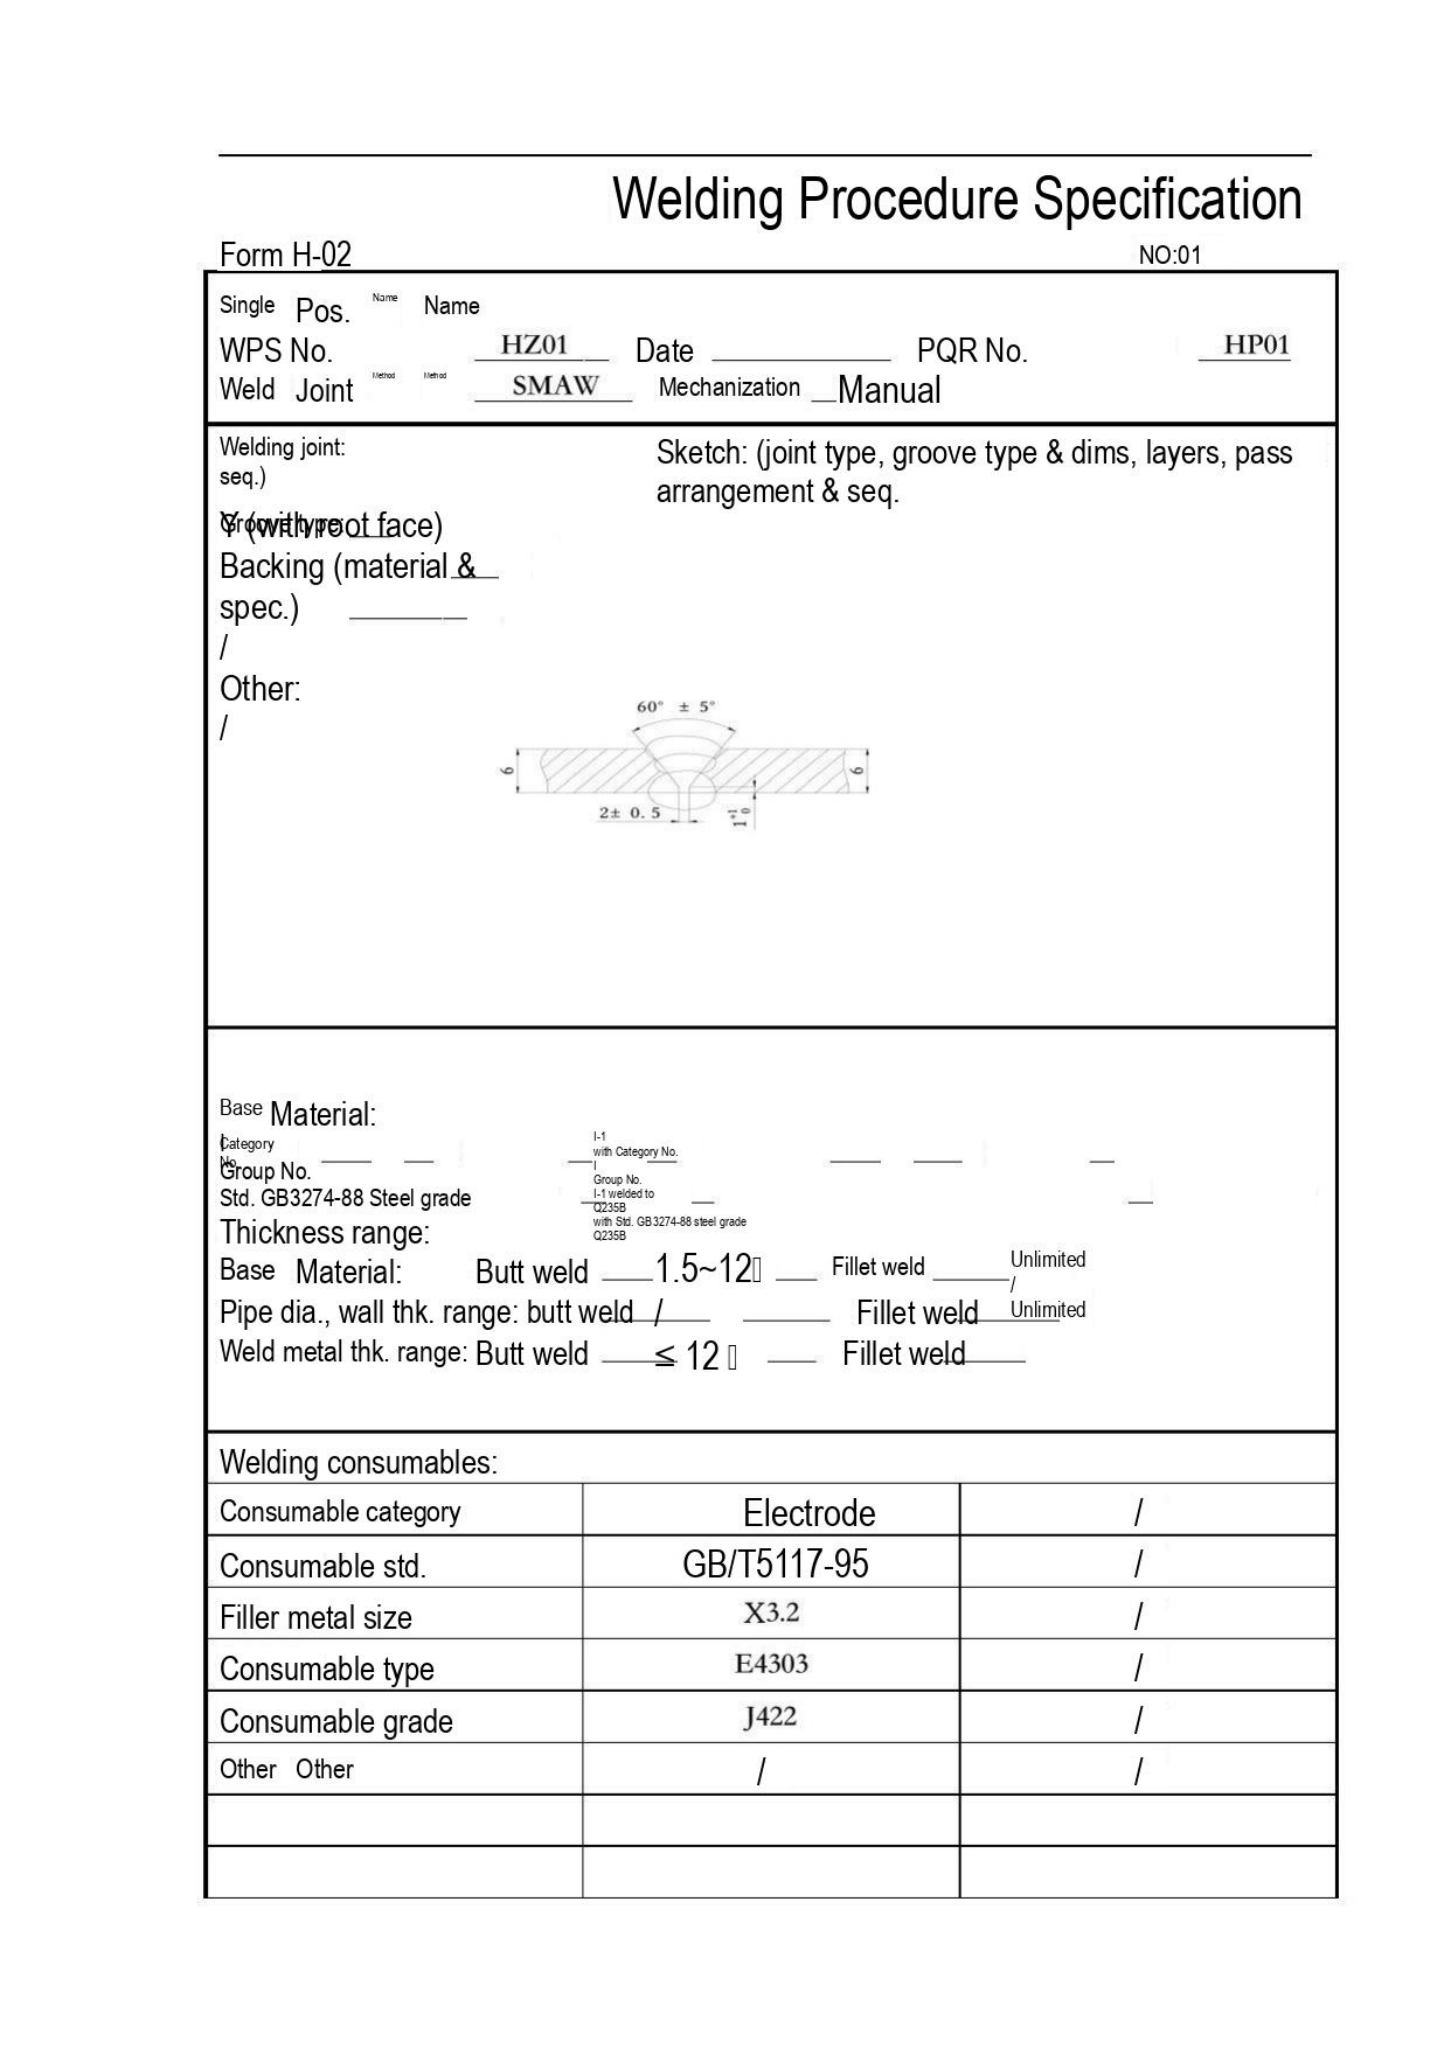Welding Procedure Specification

Form H-02 NO:01

Single Pos. Name Name
WPS No. HZ01 Date PQR No. HP01
Weld Joint Method Method SMAW Mechanization Manual

Welding joint: Sketch: (joint type, groove type & dims, layers, pass arrangement & seq.)
seq.)
Groove type: Y (with root face)
Backing (material & spec.)
/
Other:
/

60° ± 5°
9
9
2± 0.5
1±0

Base Material:
Category No. I-1 with Category No. I
Group No. Group No. I-1 welded to Q235B
Std. GB3274-88 Steel grade with Std. GB3274-88 steel grade Q235B
Thickness range:
Base Material: Butt weld 1.5~12 Fillet weld Unlimited
/
Pipe dia., wall thk. range: butt weld / Fillet weld Unlimited
Weld metal thk. range: Butt weld ≤ 12 Fillet weld

Welding consumables:

| Consumable category | Electrode | / |
|---|---|---|
| Consumable std. | GB/T5117-95 | / |
| Filler metal size | X3.2 | / |
| Consumable type | E4303 | / |
| Consumable grade | J422 | / |
| Other Other | / | / |
| | | |
| | | |
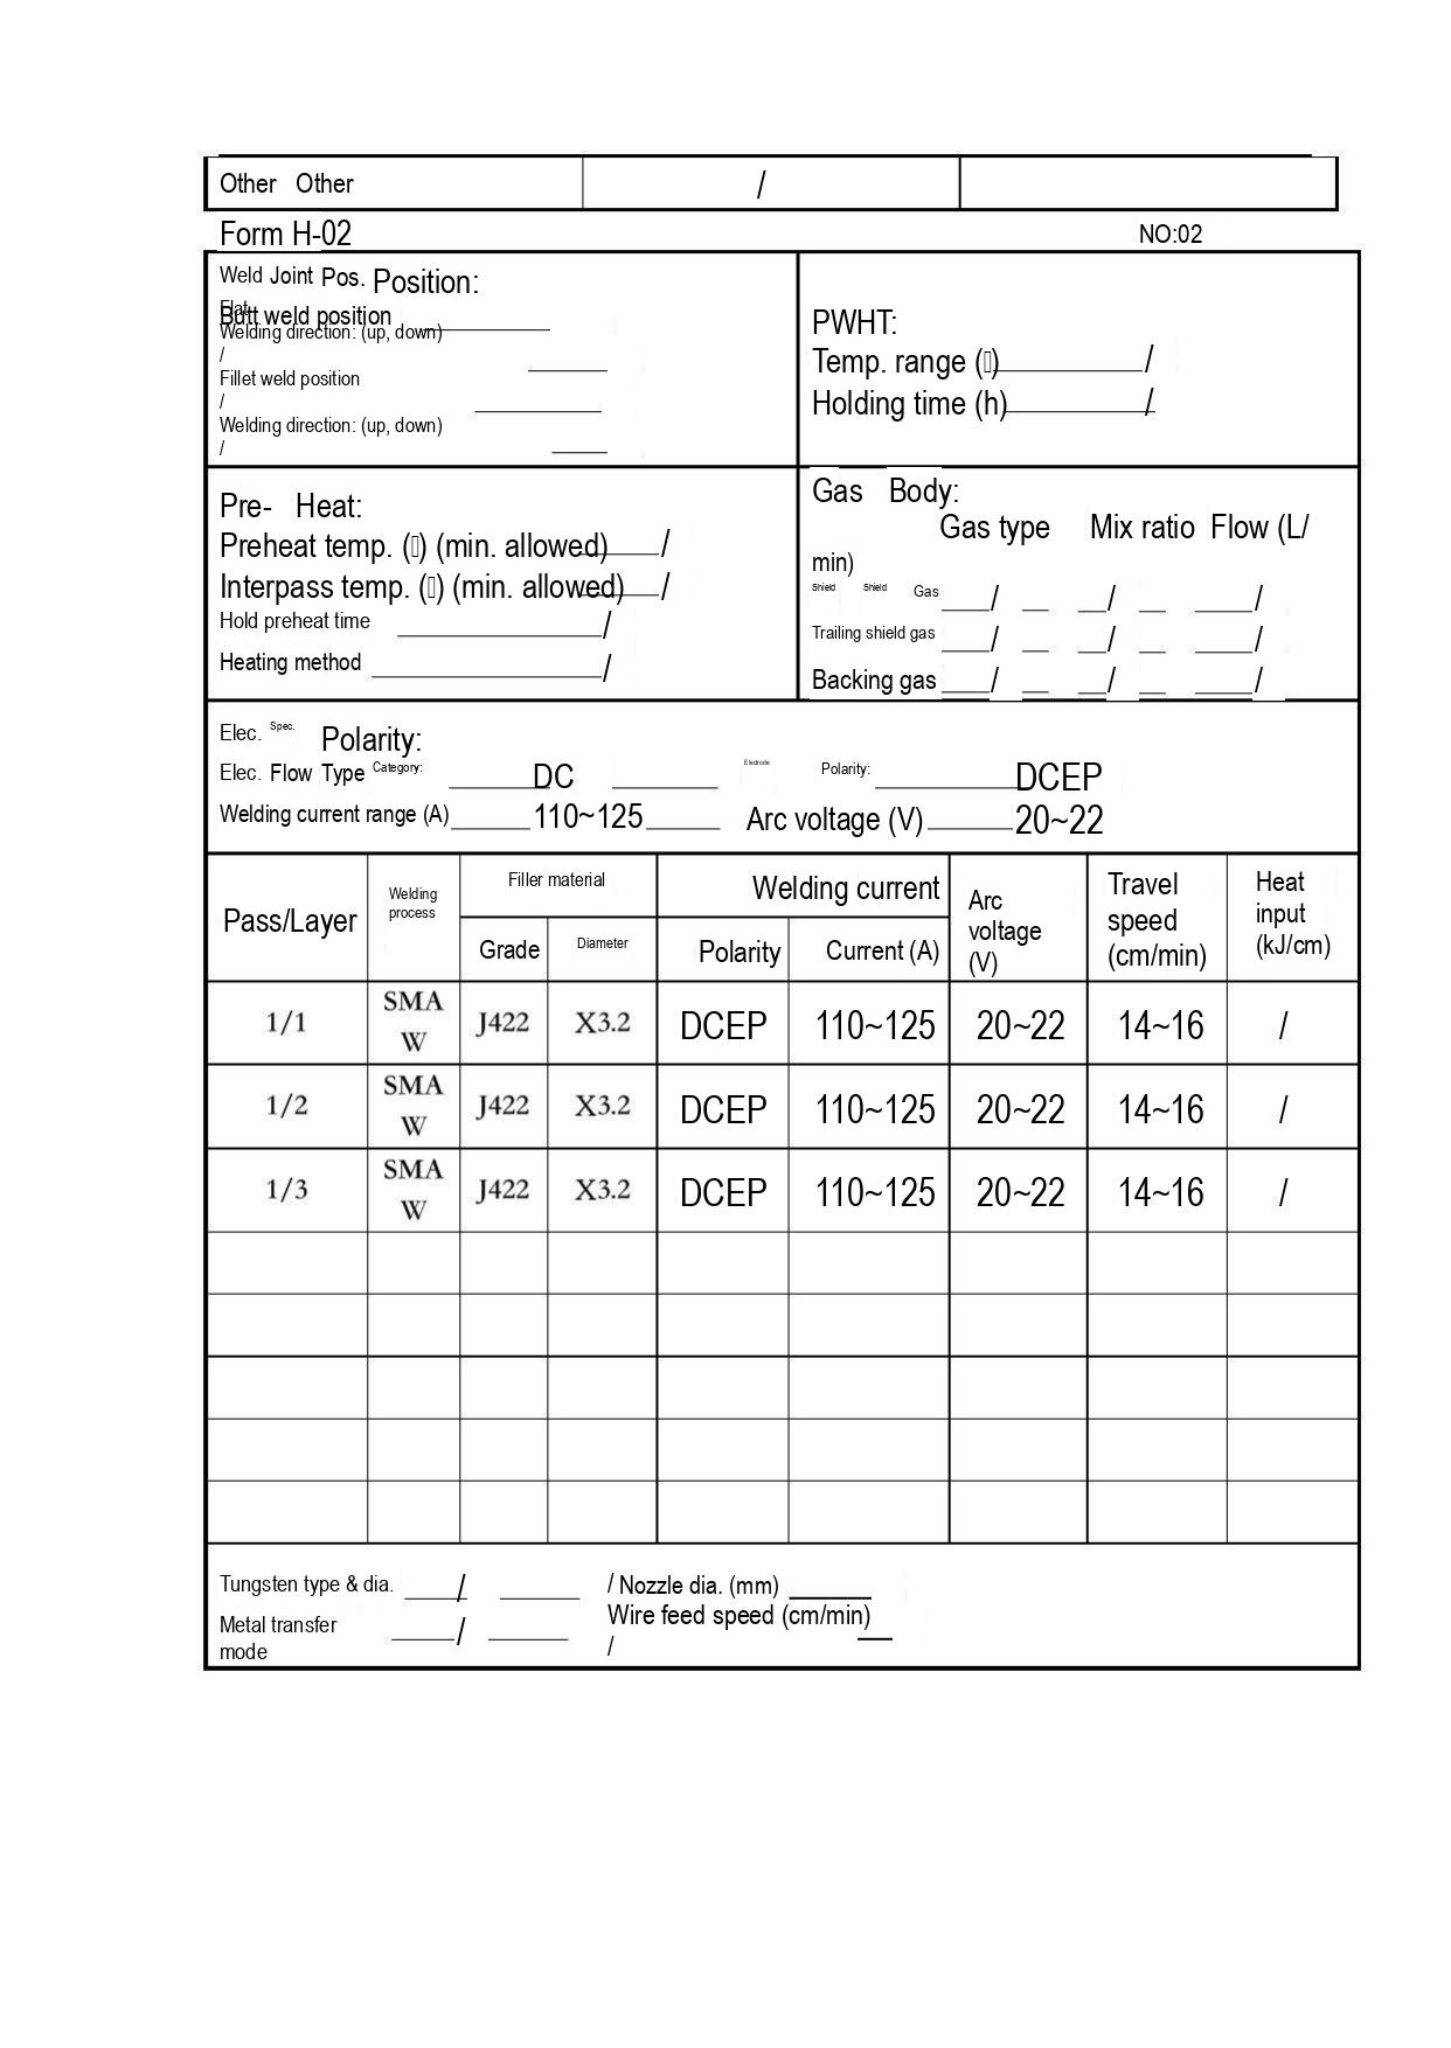| Other Other | / | |
|---|---|---|

Form H-02 NO:02

| Weld Joint Pos. Position:<br>Flat<br>Butt weld position<br>Welding direction: (up, down)<br>/<br>Fillet weld position<br>/<br>Welding direction: (up, down)<br>/ | PWHT:<br>Temp. range (℃) /<br>Holding time (h) / |
|---|---|
| Pre- Heat:<br>Preheat temp. (℃) (min. allowed) /<br>Interpass temp. (℃) (min. allowed) /<br>Hold preheat time /<br>Heating method / | Gas Body:<br>Gas type Mix ratio Flow (L/min)<br>Shield Shield Gas / / /<br>Trailing shield gas / / /<br>Backing gas / / / |

Elec. Spec. Polarity:
Elec. Flow Type Category: DC Electrode Polarity: DCEP
Welding current range (A) 110~125 Arc voltage (V) 20~22

| Pass/Layer | Welding process | Filler material Grade | Filler material Diameter | Welding current Polarity | Welding current Current (A) | Arc voltage (V) | Travel speed (cm/min) | Heat input (kJ/cm) |
|---|---|---|---|---|---|---|---|---|
| 1/1 | SMAW | J422 | X3.2 | DCEP | 110~125 | 20~22 | 14~16 | / |
| 1/2 | SMAW | J422 | X3.2 | DCEP | 110~125 | 20~22 | 14~16 | / |
| 1/3 | SMAW | J422 | X3.2 | DCEP | 110~125 | 20~22 | 14~16 | / |
| | | | | | | | | |
| | | | | | | | | |
| | | | | | | | | |
| | | | | | | | | |
| | | | | | | | | |

Tungsten type & dia. / / Nozzle dia. (mm)
Metal transfer mode / Wire feed speed (cm/min) /
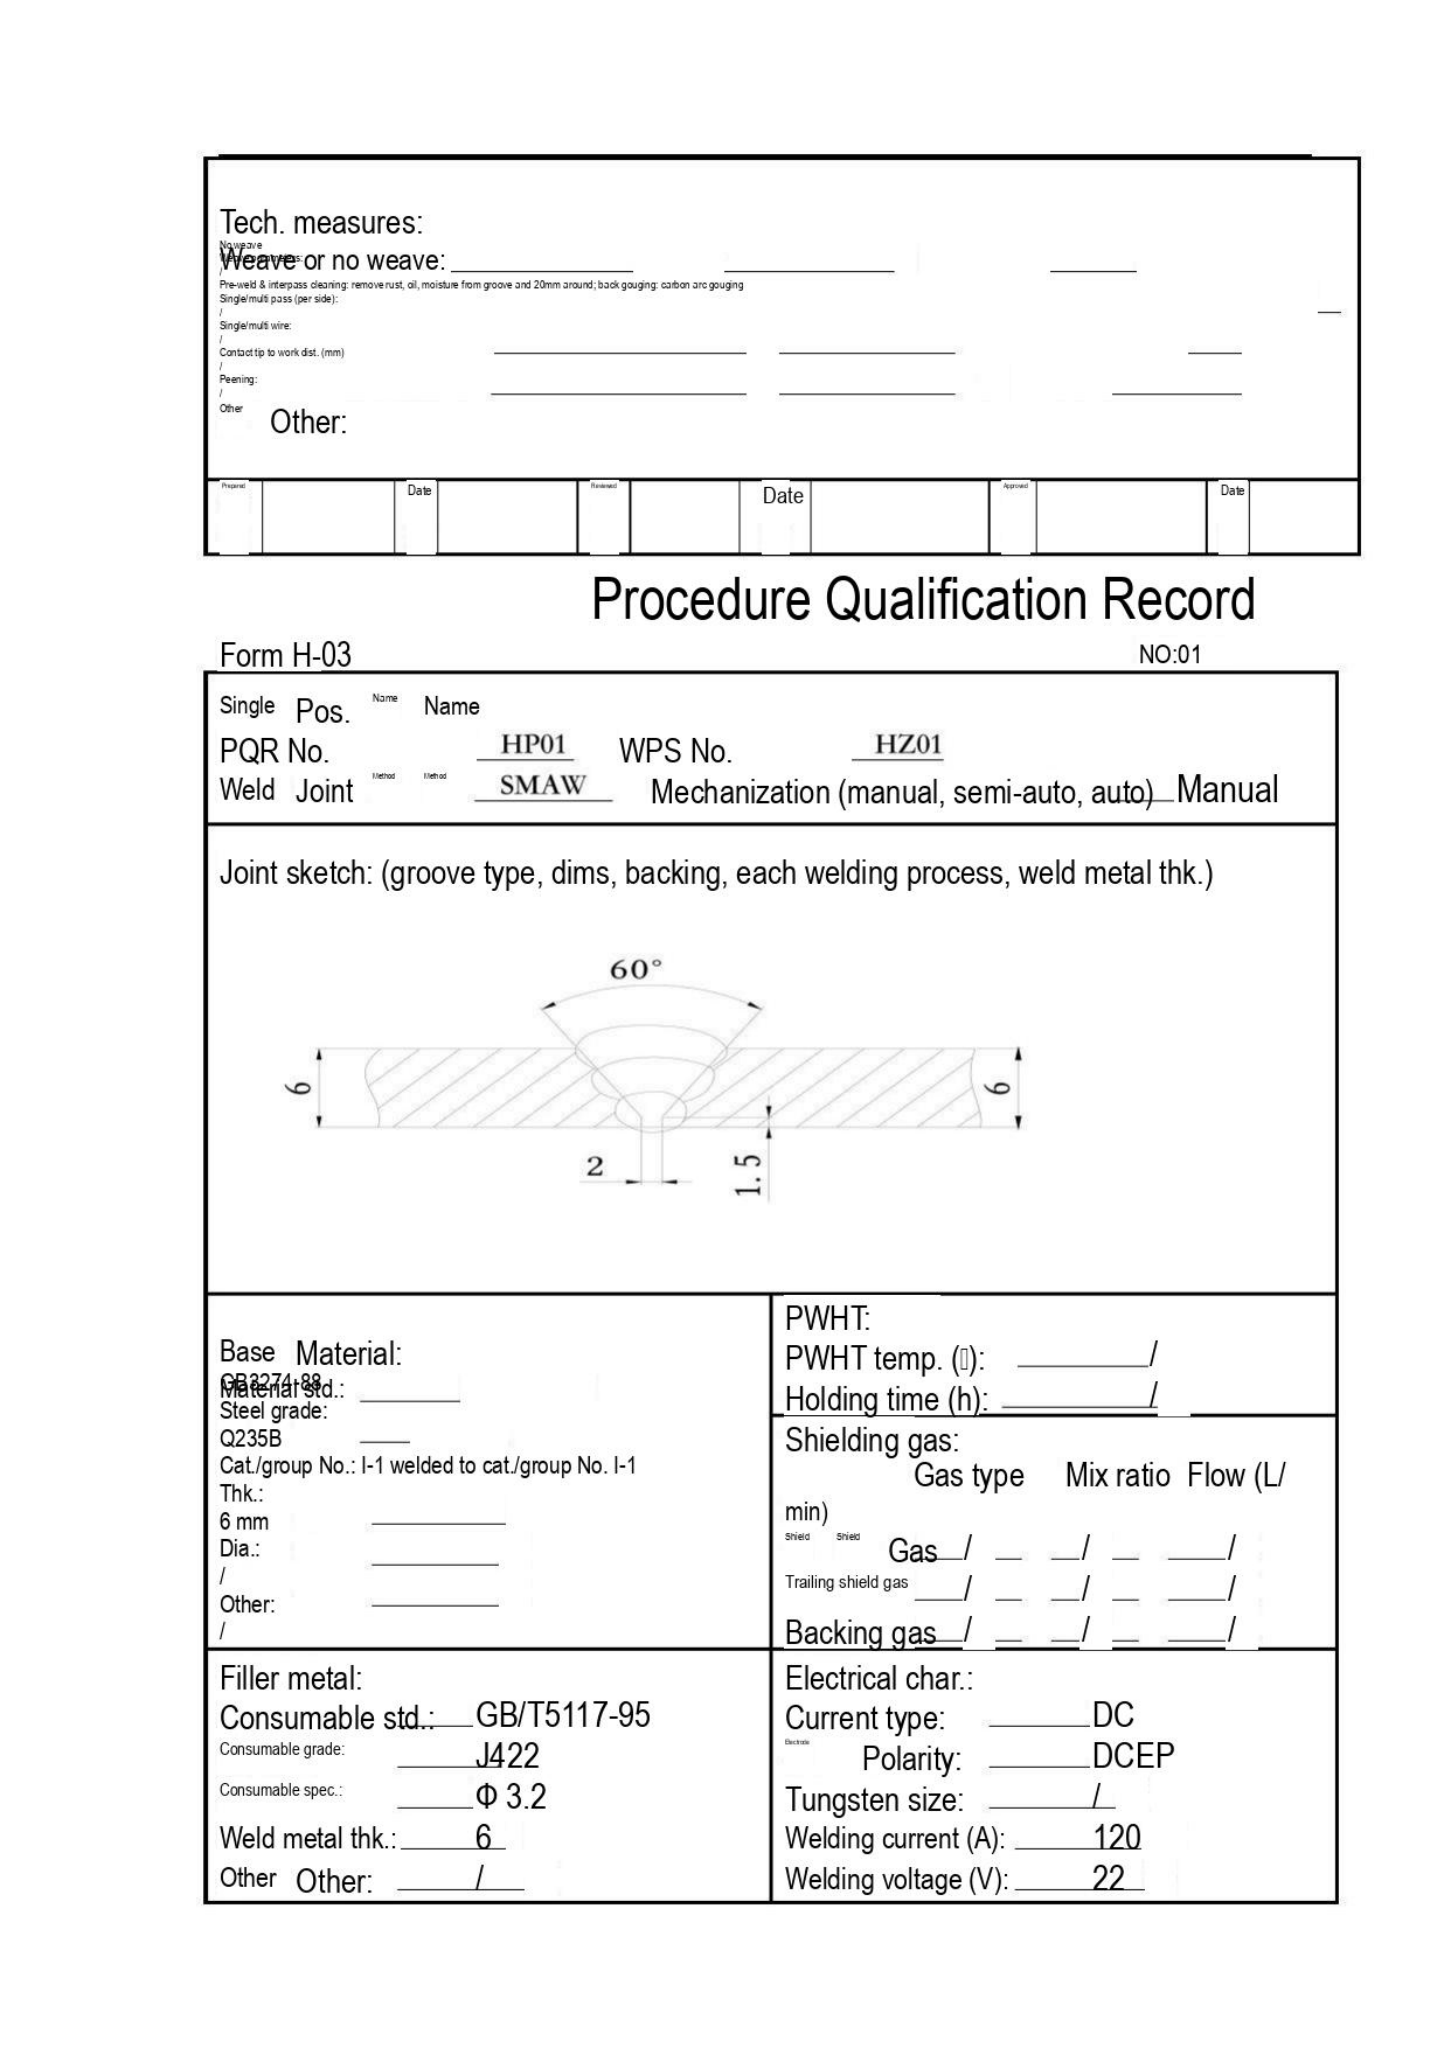Tech. measures:
No weave
Weave or no weave:
Pre-weld & interpass cleaning: remove rust, oil, moisture from groove and 20mm around; back gouging: carbon arc gouging
Single/multi pass (per side):
/
Single/multi wire:
/
Contact tip to work dist. (mm)
/
Peening:
/
Other
Other:

| Prepared | | Date | | Reviewed | | Date | | Approved | | Date | |
|---|---|---|---|---|---|---|---|---|---|---|---|

Procedure Qualification Record

Form H-03 NO:01

Single Pos. Name Name
PQR No. HP01 WPS No. HZ01
Weld Joint Method Method SMAW Mechanization (manual, semi-auto, auto) Manual

Joint sketch: (groove type, dims, backing, each welding process, weld metal thk.)

60°
6
6
2
1.5

| Base Material:<br>GB3274-88<br>Material std.:<br>Steel grade:<br>Q235B<br>Cat./group No.: I-1 welded to cat./group No. I-1<br>Thk.:<br>6 mm<br>Dia.:<br>/<br>Other:<br>/ | PWHT:<br>PWHT temp. (℃): /<br>Holding time (h): /<br><br>Shielding gas:<br>Gas type Mix ratio Flow (L/min)<br>Shield Shield Gas / / /<br>Trailing shield gas / / /<br>Backing gas / / / |
|---|---|
| Filler metal:<br>Consumable std.: GB/T5117-95<br>Consumable grade: J422<br>Consumable spec.: Φ 3.2<br>Weld metal thk.: 6<br>Other Other: / | Electrical char.:<br>Current type: DC<br>Electrode Polarity: DCEP<br>Tungsten size: /<br>Welding current (A): 120<br>Welding voltage (V): 22 |
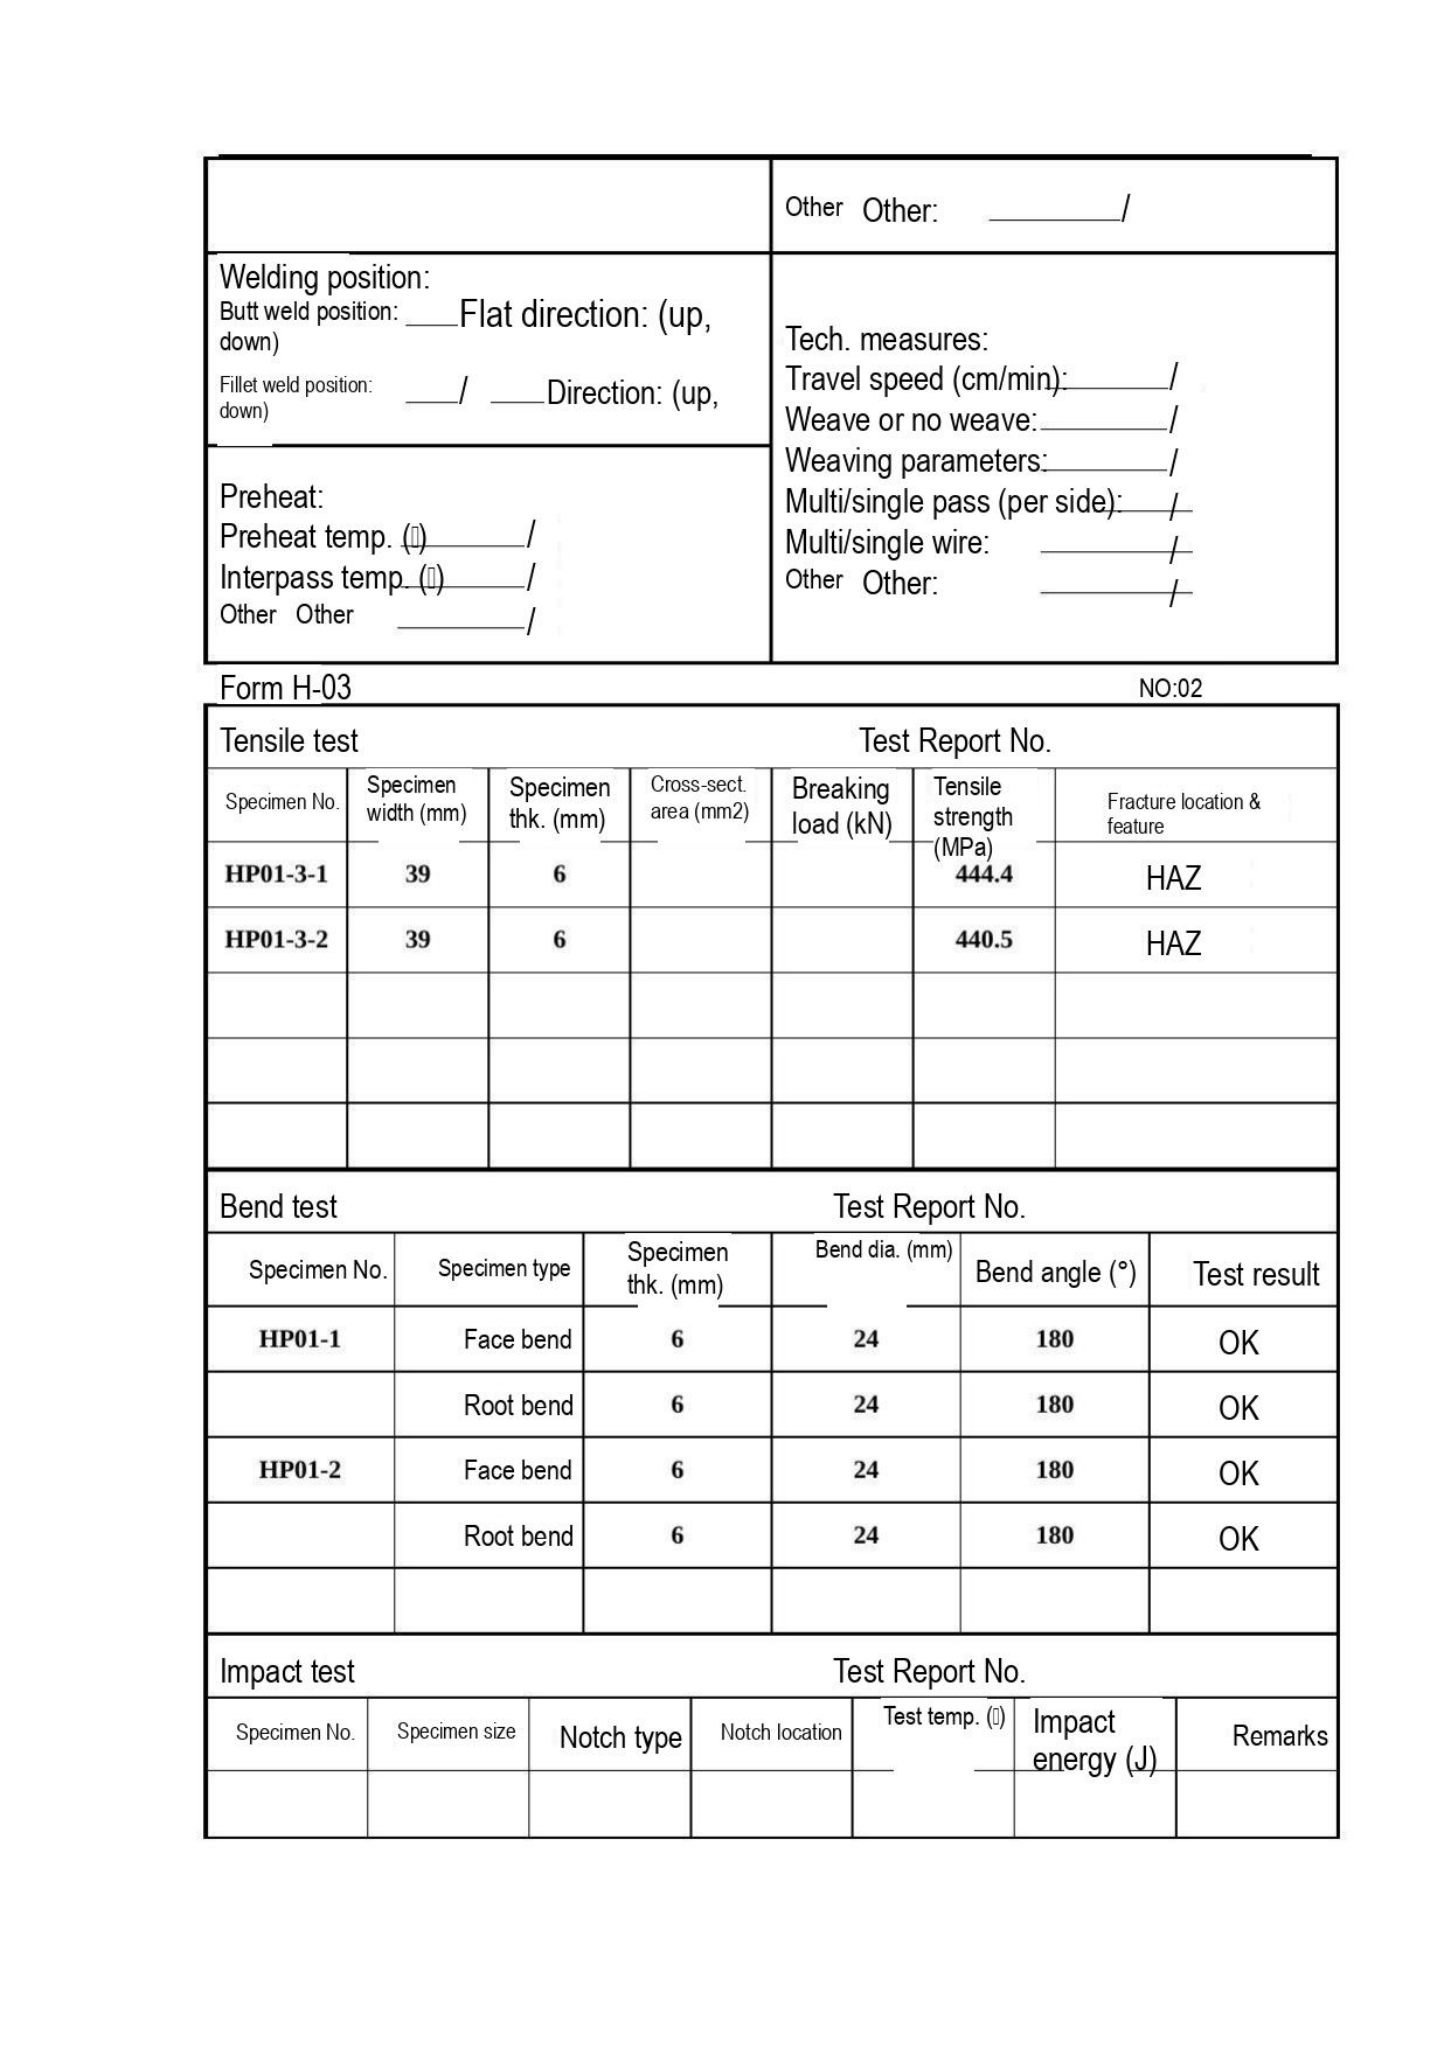| | |
|---|---|
| | Other Other: _________/ |
| Welding position:<br>Butt weld position: ____Flat direction: (up, down)<br>Fillet weld position: ____/ ____Direction: (up, down) | Tech. measures:<br>Travel speed (cm/min):________/<br>Weave or no weave:________/<br>Weaving parameters:________/<br>Multi/single pass (per side):__/<br>Multi/single wire: ________/<br>Other Other: ________/ |
| Preheat:<br>Preheat temp. ()________/<br>Interpass temp. ()________/<br>Other Other _________/ | |

Form H-03 NO:02

**Tensile test** Test Report No.

| Specimen No. | Specimen width (mm) | Specimen thk. (mm) | Cross-sect. area (mm2) | Breaking load (kN) | Tensile strength (MPa) | Fracture location & feature |
|---|---|---|---|---|---|---|
| HP01-3-1 | 39 | 6 | | | 444.4 | HAZ |
| HP01-3-2 | 39 | 6 | | | 440.5 | HAZ |
| | | | | | | |
| | | | | | | |
| | | | | | | |

**Bend test** Test Report No.

| Specimen No. | Specimen type | Specimen thk. (mm) | Bend dia. (mm) | Bend angle (°) | Test result |
|---|---|---|---|---|---|
| HP01-1 | Face bend | 6 | 24 | 180 | OK |
| | Root bend | 6 | 24 | 180 | OK |
| HP01-2 | Face bend | 6 | 24 | 180 | OK |
| | Root bend | 6 | 24 | 180 | OK |
| | | | | | |

**Impact test** Test Report No.

| Specimen No. | Specimen size | Notch type | Notch location | Test temp. () | Impact energy (J) | Remarks |
|---|---|---|---|---|---|---|
| | | | | | | |
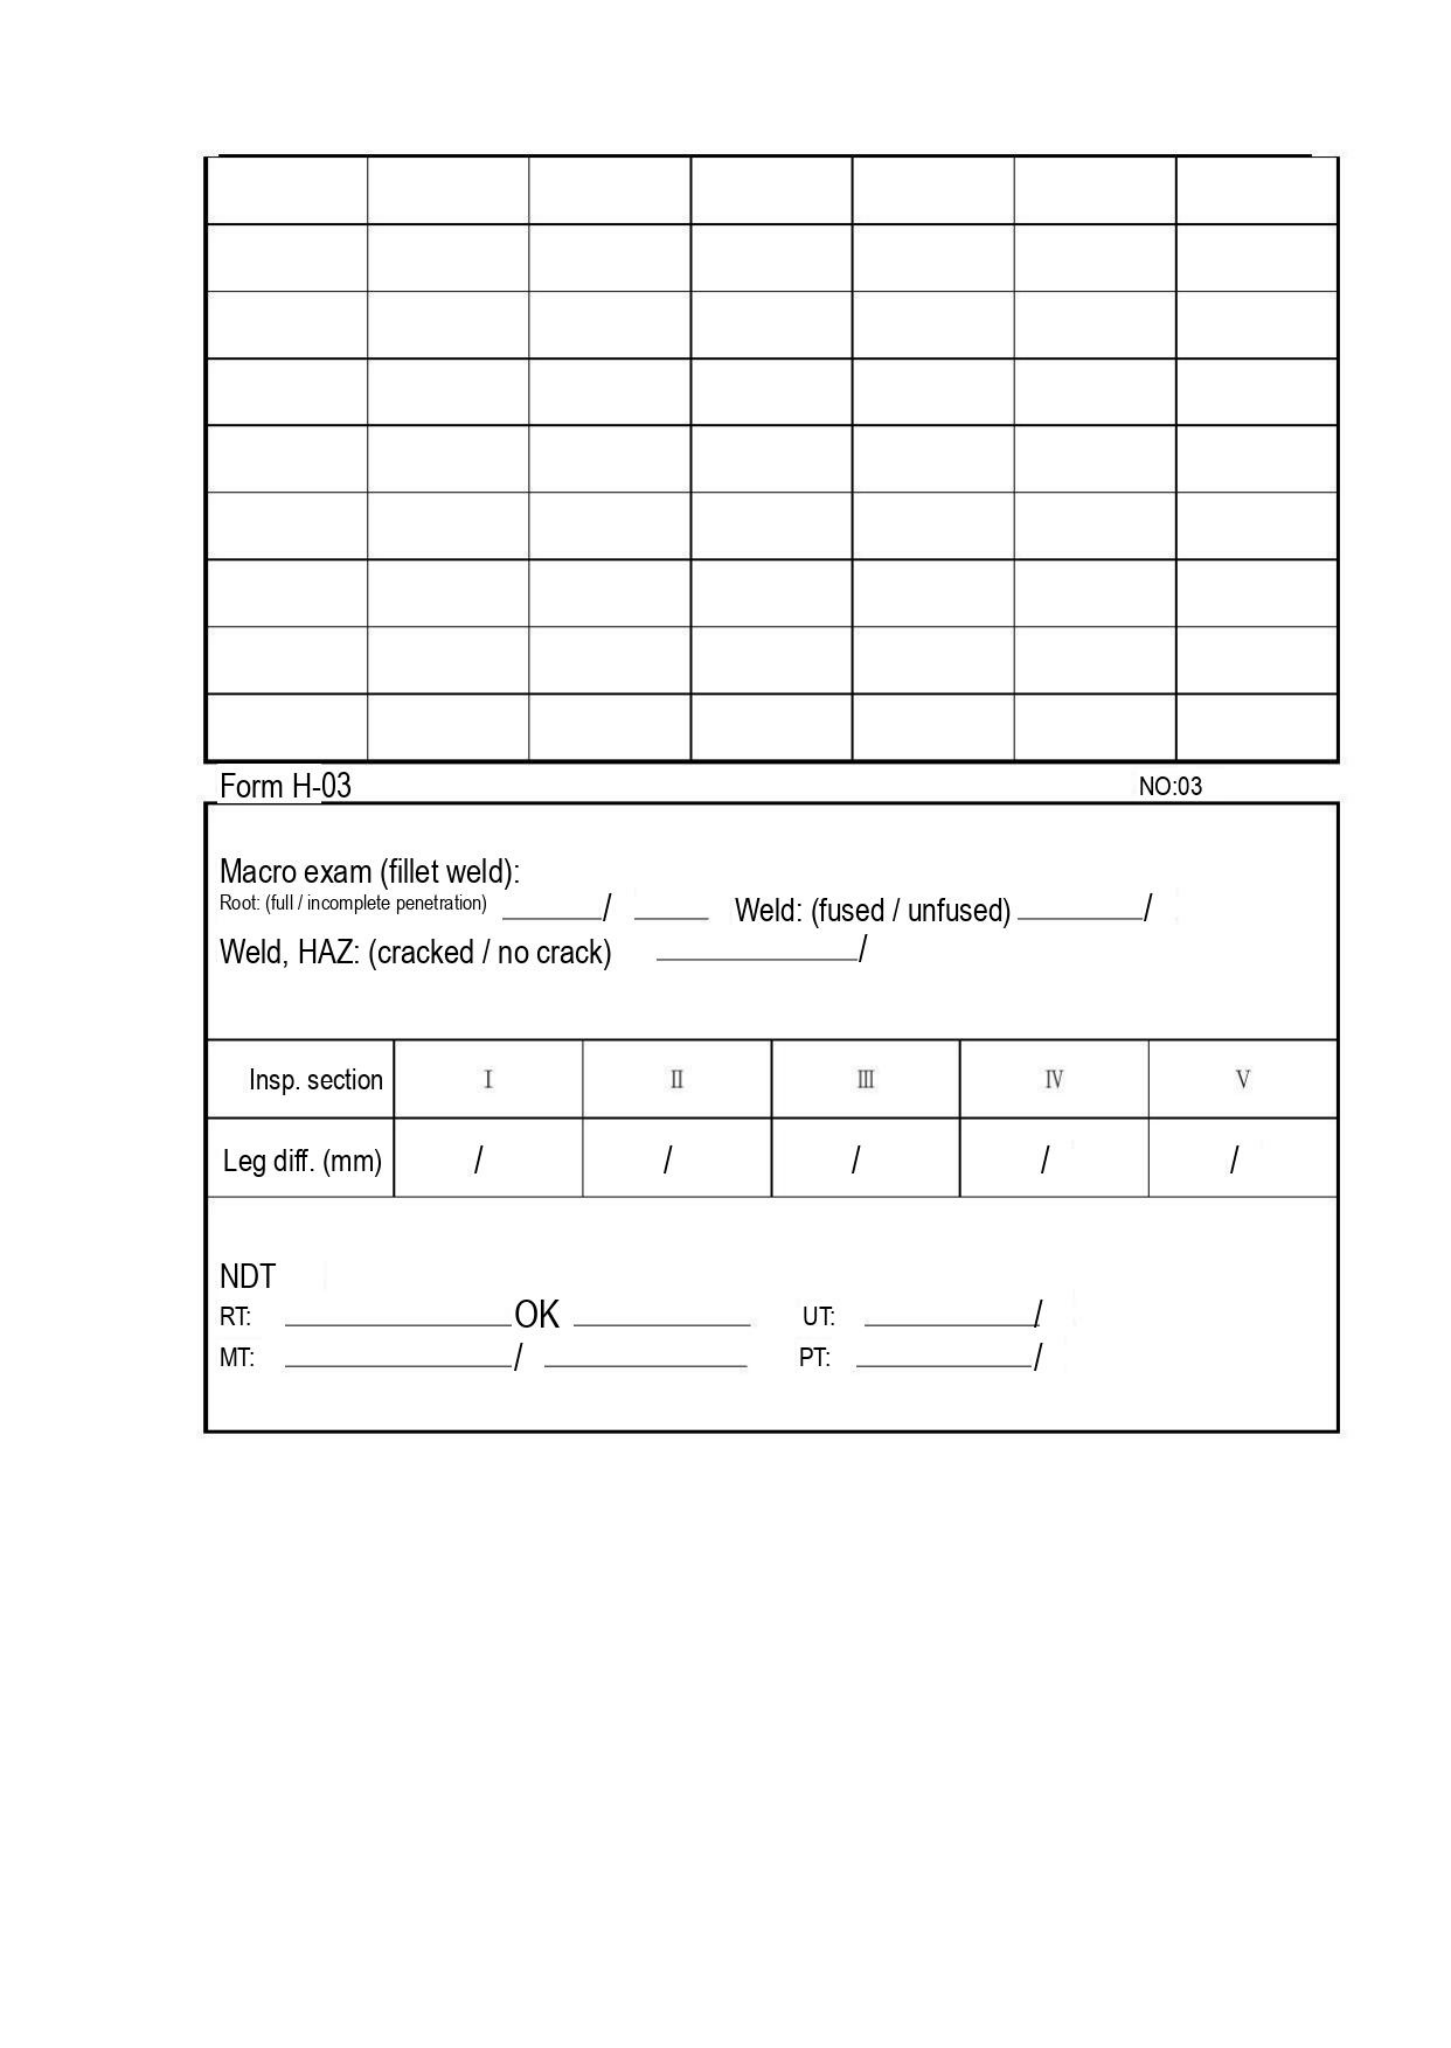|  |  |  |  |  |  |  |
|---|---|---|---|---|---|---|
|  |  |  |  |  |  |  |
|  |  |  |  |  |  |  |
|  |  |  |  |  |  |  |
|  |  |  |  |  |  |  |
|  |  |  |  |  |  |  |
|  |  |  |  |  |  |  |
|  |  |  |  |  |  |  |
|  |  |  |  |  |  |  |
|  |  |  |  |  |  |  |

Form H-03 NO:03

Macro exam (fillet weld):
Root: (full / incomplete penetration) ________/ ______ Weld: (fused / unfused) _________/
Weld, HAZ: (cracked / no crack) ____________/

| Insp. section | I | II | III | IV | V |
|---|---|---|---|---|---|
| Leg diff. (mm) | / | / | / | / | / |

NDT
RT: ______________OK ____________ UT: ___________/
MT: ______________/ ____________ PT: ___________/
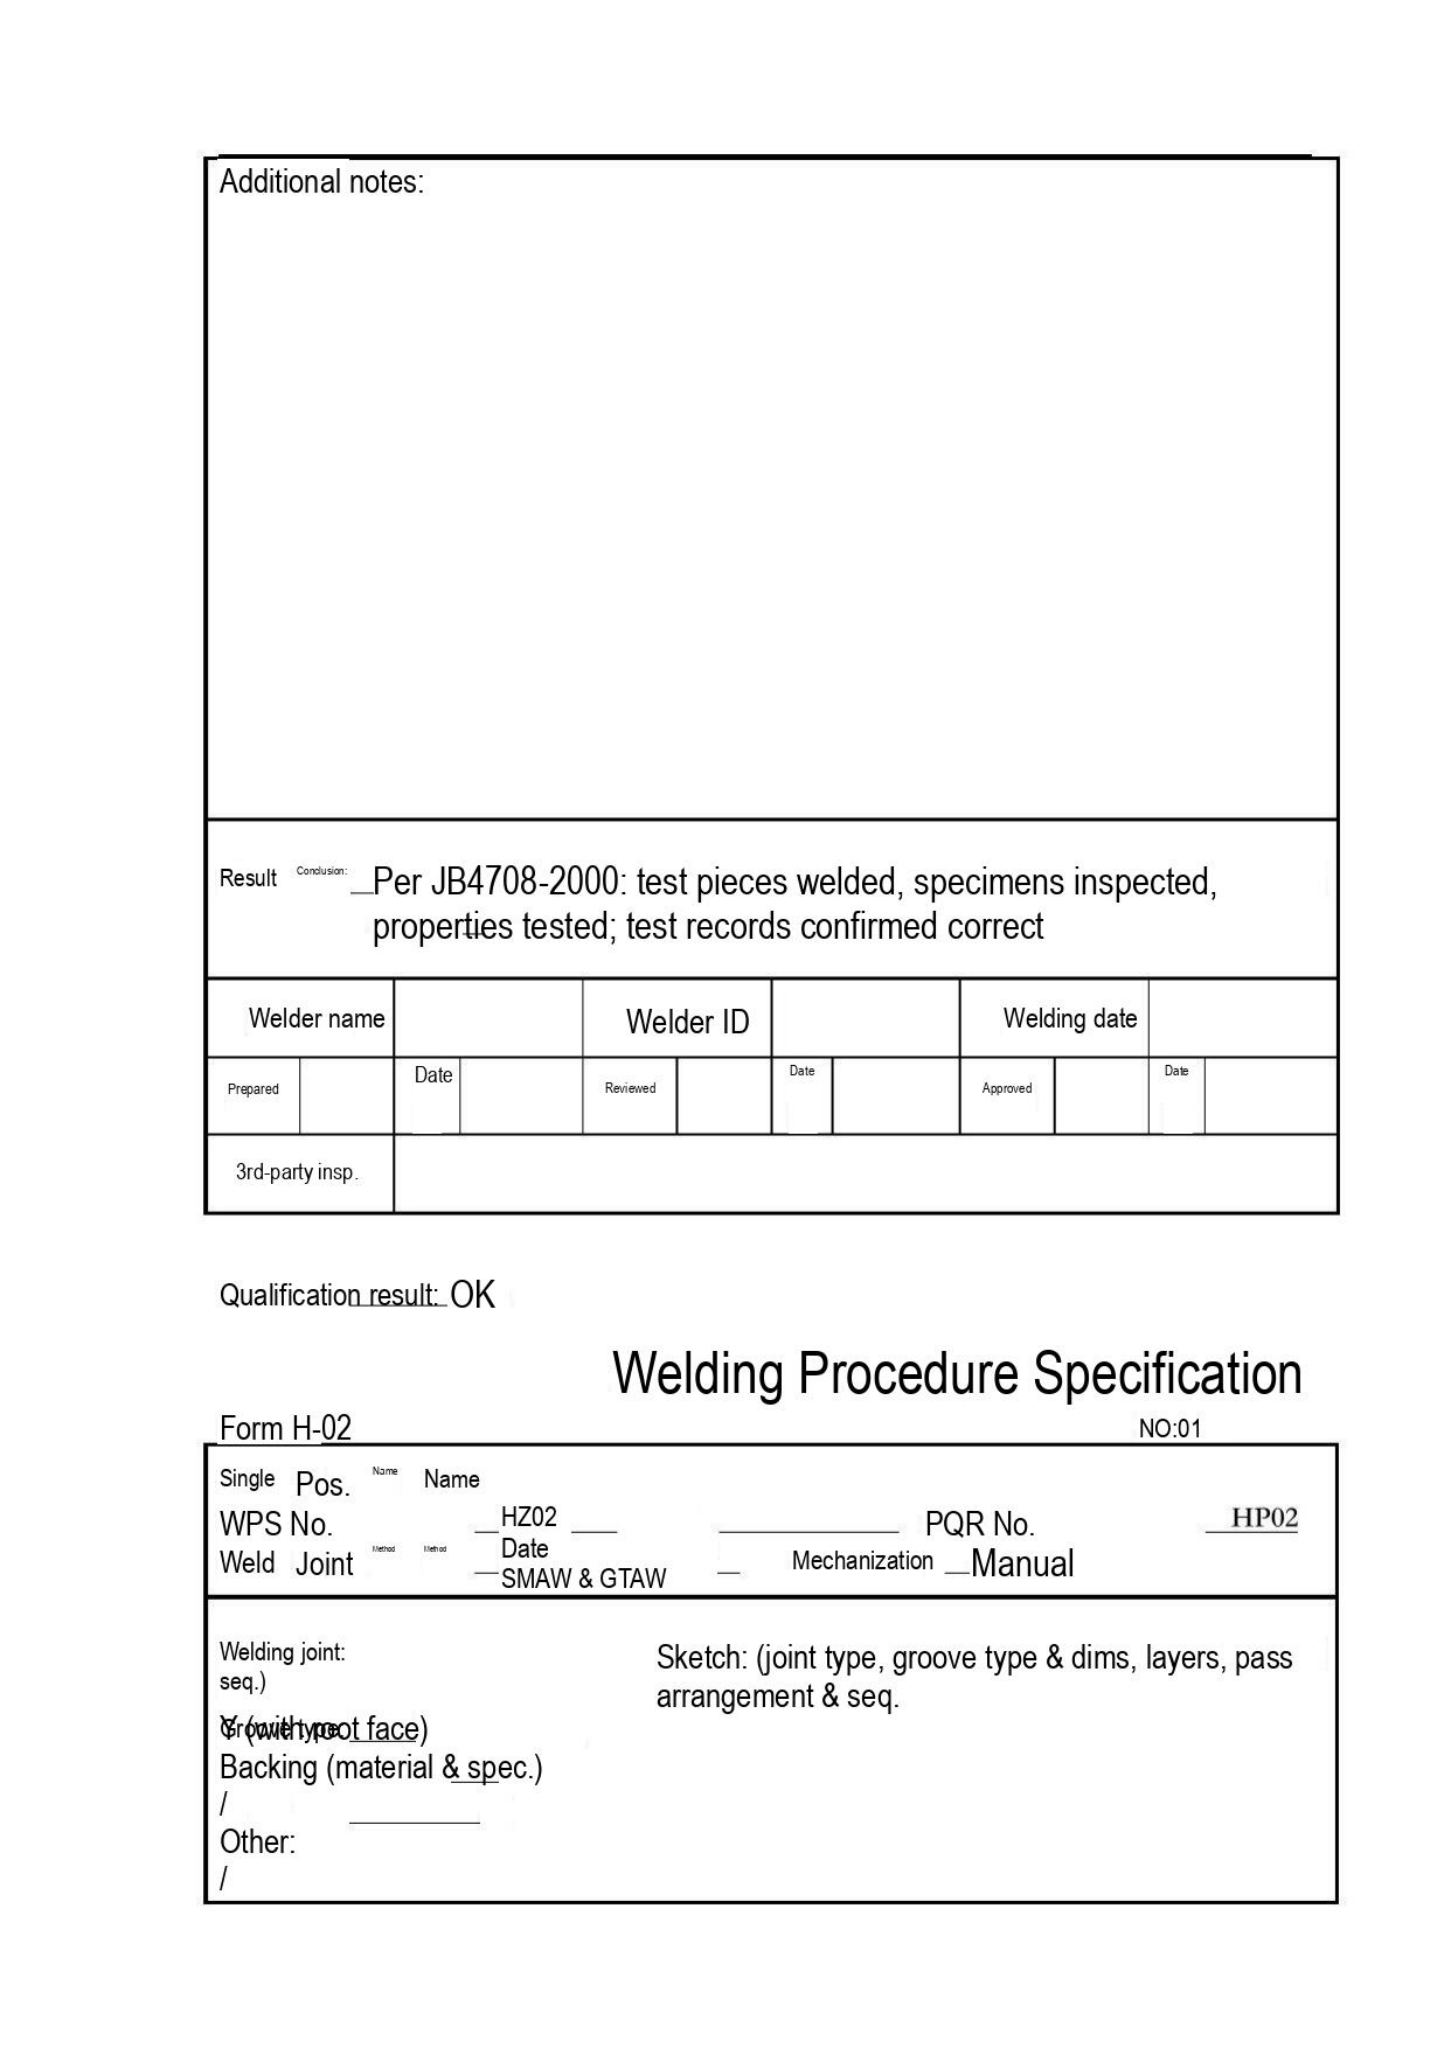Additional notes:

Result Conclusion: Per JB4708-2000: test pieces welded, specimens inspected, properties tested; test records confirmed correct

| Welder name | | Welder ID | | Welding date | |
|---|---|---|---|---|---|
| Prepared | | Date | | Reviewed | | Date | | Approved | | Date | |
| 3rd-party insp. | | | | | |

Qualification result: OK

Welding Procedure Specification

Form H-02 NO:01

Single Pos. Name Name
WPS No. HZ02 PQR No. HP02
Weld Joint Method Method Date SMAW & GTAW Mechanization Manual

Welding joint:
seq.)
Groove type Y (with root face)
Backing (material & spec.)
/
Other:
/

Sketch: (joint type, groove type & dims, layers, pass arrangement & seq.
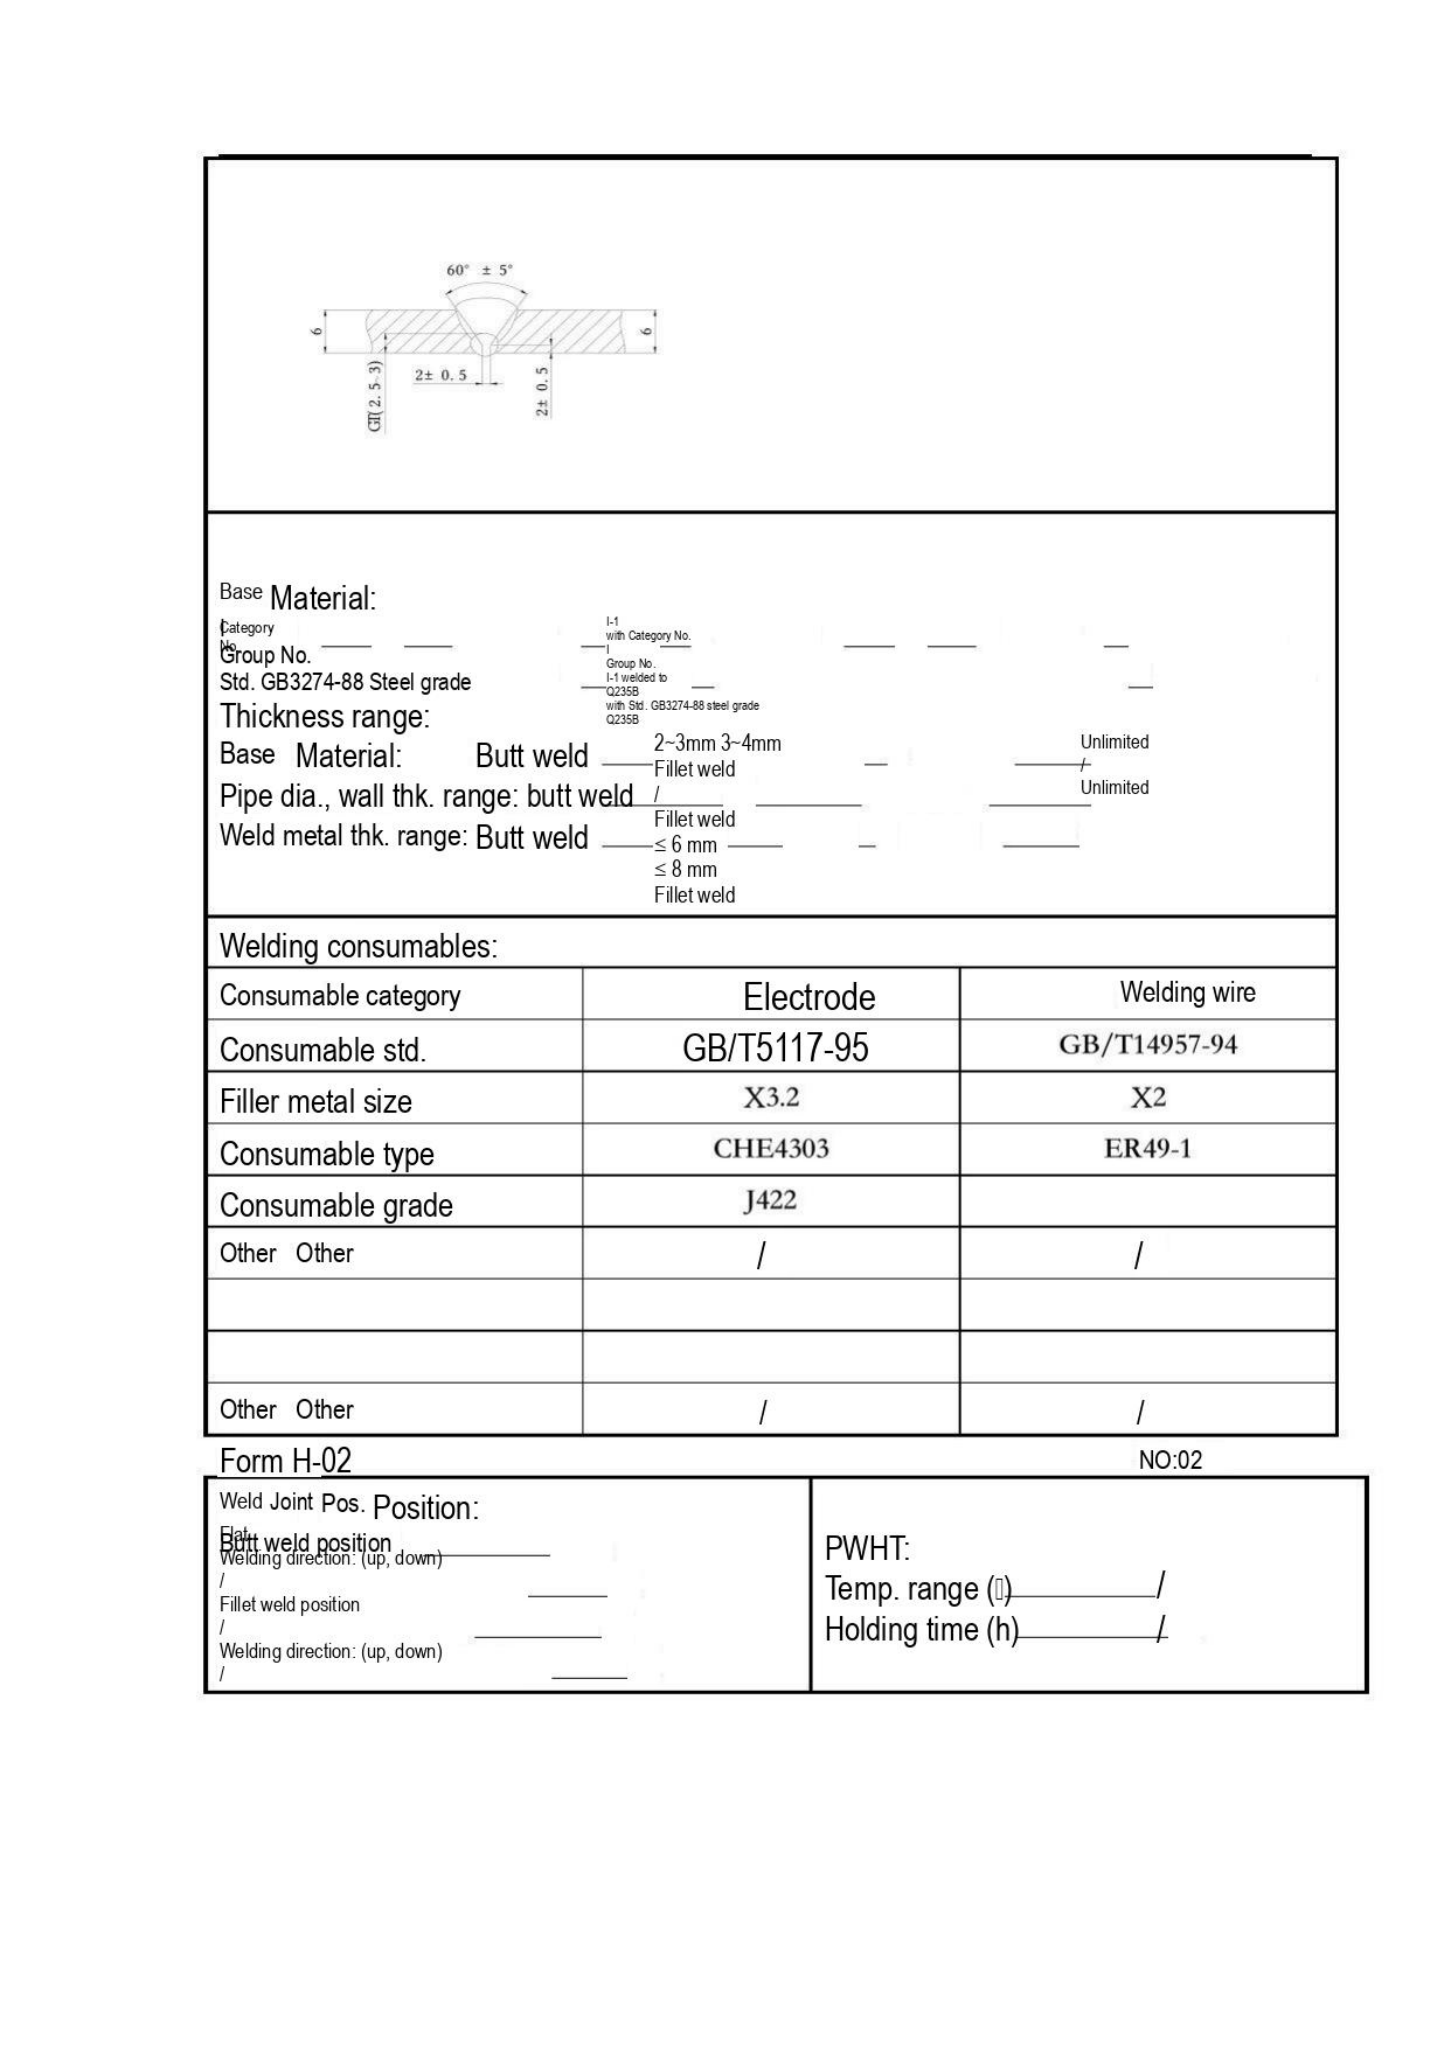60° ± 5°

6

6

2± 0.5

2± 0.5

间(2.5-3)

Base Material:

Category No.

Group No.

Std. GB3274-88 Steel grade

I-1
with Category No.
I
Group No.
I-1 welded to
Q235B
with Std. GB3274-88 steel grade
Q235B

Thickness range:

Base Material: Butt weld 2~3mm 3~4mm Unlimited

Fillet weld /

Pipe dia., wall thk. range: butt weld / Unlimited

Fillet weld

Weld metal thk. range: Butt weld ≤ 6 mm

≤ 8 mm

Fillet weld

Welding consumables:

| Consumable category | Electrode | Welding wire |
|---|---|---|
| Consumable std. | GB/T5117-95 | GB/T14957-94 |
| Filler metal size | X3.2 | X2 |
| Consumable type | CHE4303 | ER49-1 |
| Consumable grade | J422 | |
| Other Other | / | / |
| | | |
| | | |
| Other Other | / | / |

Form H-02 NO:02

| Weld Joint Pos. Position:<br>Flat<br>Butt weld position<br>Welding direction: (up, down)<br>/<br>Fillet weld position<br>/<br>Welding direction: (up, down)<br>/ | PWHT:<br>Temp. range () /<br>Holding time (h) / |
|---|---|